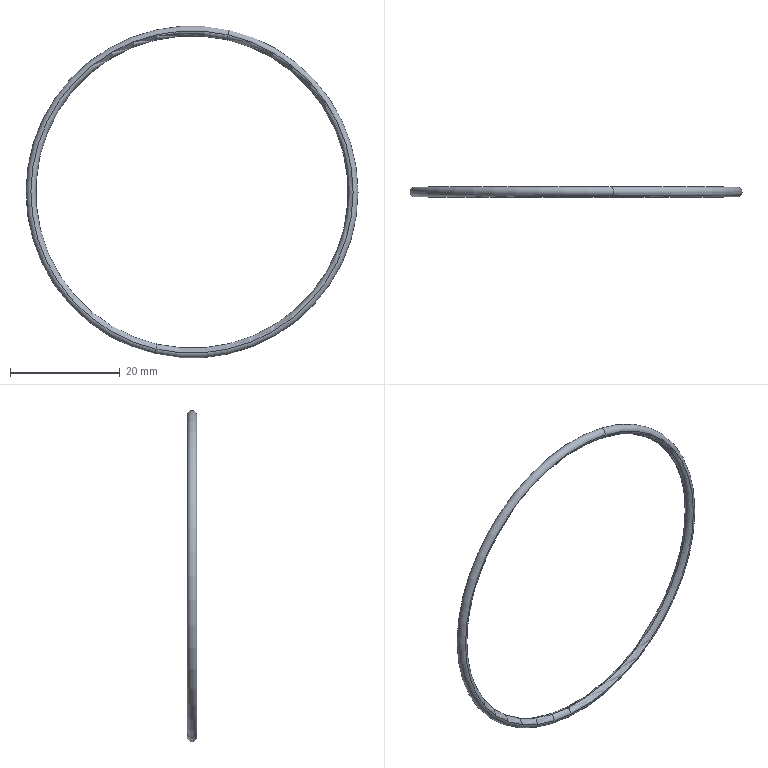Part | SolidWorks | features BaseBody 1 | 1 solid | 6 faces | box 60.43 x 1.78 x 60.43 mm | volume 458.509 mm3 | torus 6
STEP:
#1=CARTESIAN_POINT('',(2024.303,149.9,801.337));
#2=VERTEX_POINT('',#1);
#3=CARTESIAN_POINT('',(2024.104,150.79,800.47));
#4=VERTEX_POINT('',#3);
#5=CARTESIAN_POINT('',(2024.104,149.9,800.47));
#6=DIRECTION('',(-0.9746,0.,0.2239));
#7=DIRECTION('',(0.,1.,0.));
#8=AXIS2_PLACEMENT_3D('',#5,#6,#7);
#9=CIRCLE('',#8,0.89);
#10=EDGE_CURVE('',#2,#4,#9,.T.);
#11=ORIENTED_EDGE('',*,*,#10,.F.);
#12=CARTESIAN_POINT('',(2037.035,149.9,856.764));
#13=VERTEX_POINT('',#12);
#14=CARTESIAN_POINT('',(2030.669,149.9,829.051));
#15=DIRECTION('',(0.,-1.,0.));
#16=DIRECTION('',(0.,0.,-1.));
#17=AXIS2_PLACEMENT_3D('',#14,#15,#16);
#18=CIRCLE('',#17,28.435);
#19=EDGE_CURVE('',#2,#13,#18,.T.);
#20=ORIENTED_EDGE('',*,*,#19,.T.);
#21=CARTESIAN_POINT('',(2037.234,150.79,857.631));
#22=VERTEX_POINT('',#21);
#23=CARTESIAN_POINT('',(2037.234,149.9,857.631));
#24=DIRECTION('',(-0.9746,0.,0.2239));
#25=DIRECTION('',(0.,1.,0.));
#26=AXIS2_PLACEMENT_3D('',#23,#24,#25);
#27=CIRCLE('',#26,0.89);
#28=EDGE_CURVE('',#22,#13,#27,.T.);
#29=ORIENTED_EDGE('',*,*,#28,.F.);
#30=CARTESIAN_POINT('',(2030.669,150.79,829.051));
#31=DIRECTION('',(0.,1.,0.));
#32=DIRECTION('',(0.2239,0.,0.9746));
#33=AXIS2_PLACEMENT_3D('',#30,#31,#32);
#34=CIRCLE('',#33,29.325);
#35=EDGE_CURVE('',#22,#4,#34,.T.);
#36=ORIENTED_EDGE('',*,*,#35,.T.);
#37=EDGE_LOOP('',(#11,#20,#29,#36));
#38=FACE_OUTER_BOUND('',#37,.T.);
#39=CARTESIAN_POINT('',(2030.669,149.9,829.051));
#40=DIRECTION('',(0.,-1.,0.));
#41=DIRECTION('',(0.2239,0.,0.9746));
#42=AXIS2_PLACEMENT_3D('',#39,#40,#41);
#43=TOROIDAL_SURFACE('',#42,29.325,0.89);
#44=ADVANCED_FACE('',(#38),#43,.T.);
#45=ORIENTED_EDGE('',*,*,#28,.T.);
#46=CARTESIAN_POINT('',(2030.669,149.9,829.051));
#47=DIRECTION('',(0.,-1.,0.));
#48=DIRECTION('',(0.,0.,-1.));
#49=AXIS2_PLACEMENT_3D('',#46,#47,#48);
#50=CIRCLE('',#49,28.435);
#51=EDGE_CURVE('',#13,#2,#50,.T.);
#52=ORIENTED_EDGE('',*,*,#51,.T.);
#53=ORIENTED_EDGE('',*,*,#10,.T.);
#54=CARTESIAN_POINT('',(2030.669,150.79,829.051));
#55=DIRECTION('',(0.,1.,0.));
#56=DIRECTION('',(0.2239,0.,0.9746));
#57=AXIS2_PLACEMENT_3D('',#54,#55,#56);
#58=CIRCLE('',#57,29.325);
#59=EDGE_CURVE('',#4,#22,#58,.T.);
#60=ORIENTED_EDGE('',*,*,#59,.T.);
#61=EDGE_LOOP('',(#45,#52,#53,#60));
#62=FACE_OUTER_BOUND('',#61,.T.);
#63=CARTESIAN_POINT('',(2030.669,149.9,829.051));
#64=DIRECTION('',(0.,-1.,0.));
#65=DIRECTION('',(0.2239,0.,0.9746));
#66=AXIS2_PLACEMENT_3D('',#63,#64,#65);
#67=TOROIDAL_SURFACE('',#66,29.325,0.89);
#68=ADVANCED_FACE('',(#62),#67,.T.);
#69=ORIENTED_EDGE('',*,*,#51,.F.);
#70=CARTESIAN_POINT('',(2037.234,149.01,857.631));
#71=VERTEX_POINT('',#70);
#72=CARTESIAN_POINT('',(2037.234,149.9,857.631));
#73=DIRECTION('',(-0.9746,0.,0.2239));
#74=DIRECTION('',(0.,1.,0.));
#75=AXIS2_PLACEMENT_3D('',#72,#73,#74);
#76=CIRCLE('',#75,0.89);
#77=EDGE_CURVE('',#13,#71,#76,.T.);
#78=ORIENTED_EDGE('',*,*,#77,.T.);
#79=CARTESIAN_POINT('',(2024.104,149.01,800.47));
#80=VERTEX_POINT('',#79);
#81=CARTESIAN_POINT('',(2030.669,149.01,829.051));
#82=DIRECTION('',(0.,-1.,0.));
#83=DIRECTION('',(0.2239,0.,0.9746));
#84=AXIS2_PLACEMENT_3D('',#81,#82,#83);
#85=CIRCLE('',#84,29.325);
#86=EDGE_CURVE('',#71,#80,#85,.T.);
#87=ORIENTED_EDGE('',*,*,#86,.T.);
#88=CARTESIAN_POINT('',(2024.104,149.9,800.47));
#89=DIRECTION('',(-0.9746,0.,0.2239));
#90=DIRECTION('',(0.,1.,0.));
#91=AXIS2_PLACEMENT_3D('',#88,#89,#90);
#92=CIRCLE('',#91,0.89);
#93=EDGE_CURVE('',#80,#2,#92,.T.);
#94=ORIENTED_EDGE('',*,*,#93,.T.);
#95=EDGE_LOOP('',(#69,#78,#87,#94));
#96=FACE_OUTER_BOUND('',#95,.T.);
#97=CARTESIAN_POINT('',(2030.669,149.9,829.051));
#98=DIRECTION('',(0.,-1.,0.));
#99=DIRECTION('',(0.2239,0.,0.9746));
#100=AXIS2_PLACEMENT_3D('',#97,#98,#99);
#101=TOROIDAL_SURFACE('',#100,29.325,0.89);
#102=ADVANCED_FACE('',(#96),#101,.T.);
#103=ORIENTED_EDGE('',*,*,#19,.F.);
#104=ORIENTED_EDGE('',*,*,#93,.F.);
#105=CARTESIAN_POINT('',(2030.669,149.01,829.051));
#106=DIRECTION('',(0.,-1.,0.));
#107=DIRECTION('',(0.2239,0.,0.9746));
#108=AXIS2_PLACEMENT_3D('',#105,#106,#107);
#109=CIRCLE('',#108,29.325);
#110=EDGE_CURVE('',#80,#71,#109,.T.);
#111=ORIENTED_EDGE('',*,*,#110,.T.);
#112=ORIENTED_EDGE('',*,*,#77,.F.);
#113=EDGE_LOOP('',(#103,#104,#111,#112));
#114=FACE_OUTER_BOUND('',#113,.T.);
#115=CARTESIAN_POINT('',(2030.669,149.9,829.051));
#116=DIRECTION('',(0.,-1.,0.));
#117=DIRECTION('',(0.2239,0.,0.9746));
#118=AXIS2_PLACEMENT_3D('',#115,#116,#117);
#119=TOROIDAL_SURFACE('',#118,29.325,0.89);
#120=ADVANCED_FACE('',(#114),#119,.T.);
#121=ORIENTED_EDGE('',*,*,#110,.F.);
#122=CARTESIAN_POINT('',(2024.104,149.9,800.47));
#123=DIRECTION('',(0.9746,0.,-0.2239));
#124=DIRECTION('',(0.,-1.,0.));
#125=AXIS2_PLACEMENT_3D('',#122,#123,#124);
#126=CIRCLE('',#125,0.89);
#127=EDGE_CURVE('',#80,#4,#126,.T.);
#128=ORIENTED_EDGE('',*,*,#127,.T.);
#129=ORIENTED_EDGE('',*,*,#35,.F.);
#130=CARTESIAN_POINT('',(2037.234,149.9,857.631));
#131=DIRECTION('',(0.9746,0.,-0.2239));
#132=DIRECTION('',(0.,-1.,0.));
#133=AXIS2_PLACEMENT_3D('',#130,#131,#132);
#134=CIRCLE('',#133,0.89);
#135=EDGE_CURVE('',#22,#71,#134,.T.);
#136=ORIENTED_EDGE('',*,*,#135,.T.);
#137=EDGE_LOOP('',(#121,#128,#129,#136));
#138=FACE_OUTER_BOUND('',#137,.T.);
#139=CARTESIAN_POINT('',(2030.669,149.9,829.051));
#140=DIRECTION('',(0.,-1.,0.));
#141=DIRECTION('',(0.2239,0.,0.9746));
#142=AXIS2_PLACEMENT_3D('',#139,#140,#141);
#143=TOROIDAL_SURFACE('',#142,29.325,0.89);
#144=ADVANCED_FACE('',(#138),#143,.T.);
#145=ORIENTED_EDGE('',*,*,#59,.F.);
#146=ORIENTED_EDGE('',*,*,#127,.F.);
#147=ORIENTED_EDGE('',*,*,#86,.F.);
#148=ORIENTED_EDGE('',*,*,#135,.F.);
#149=EDGE_LOOP('',(#145,#146,#147,#148));
#150=FACE_OUTER_BOUND('',#149,.T.);
#151=CARTESIAN_POINT('',(2030.669,149.9,829.051));
#152=DIRECTION('',(0.,-1.,0.));
#153=DIRECTION('',(0.2239,0.,0.9746));
#154=AXIS2_PLACEMENT_3D('',#151,#152,#153);
#155=TOROIDAL_SURFACE('',#154,29.325,0.89);
#156=ADVANCED_FACE('',(#150),#155,.T.);
#157=CLOSED_SHELL('',(#44,#68,#102,#120,#144,#156));
#158=MANIFOLD_SOLID_BREP('',#157);
#159=CARTESIAN_POINT('',(0.,0.,0.));
#160=DIRECTION('',(0.,0.,1.));
#161=DIRECTION('',(1.,0.,0.));
#162=AXIS2_PLACEMENT_3D('',#159,#160,#161);
#163=(LENGTH_UNIT()NAMED_UNIT(*)SI_UNIT(.MILLI.,.METRE.));
#164=UNCERTAINTY_MEASURE_WITH_UNIT(LENGTH_MEASURE(0.00001),#163,'','');
#165=(NAMED_UNIT(*)PLANE_ANGLE_UNIT()SI_UNIT($,.RADIAN.));
#166=(NAMED_UNIT(*)SI_UNIT($,.STERADIAN.)SOLID_ANGLE_UNIT());
#167=(GEOMETRIC_REPRESENTATION_CONTEXT(3)GLOBAL_UNCERTAINTY_ASSIGNED_CONTEXT((#164))GLOBAL_UNIT_ASSIGNED_CONTEXT((#163,#165,#166))REPRESENTATION_CONTEXT('',''));
#168=ADVANCED_BREP_SHAPE_REPRESENTATION('',(#158,#162),#167);